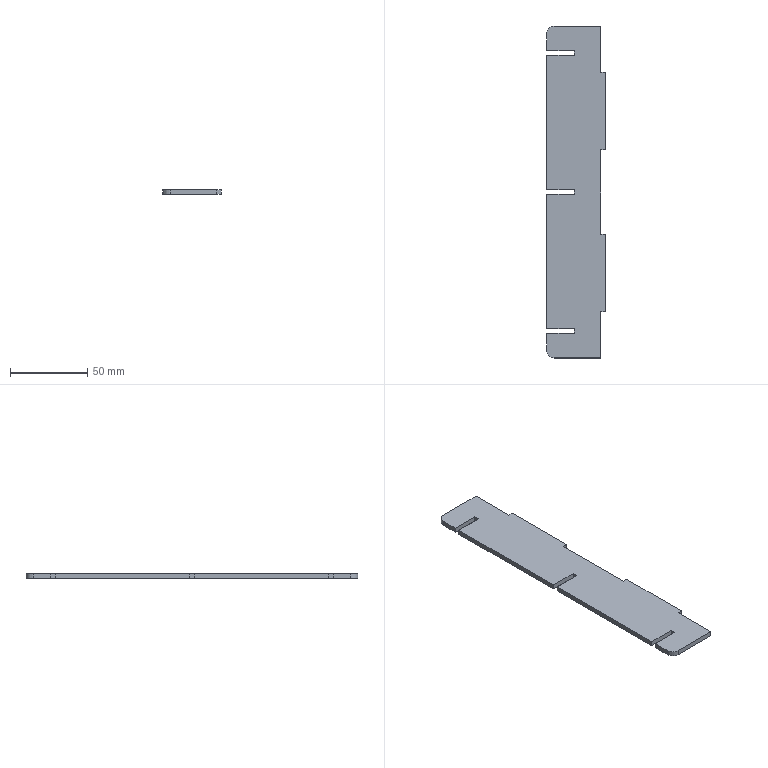Part | SolidWorks | features FlatPattern 1, SMBaseFlange 1, SheetMetal 1 | 1 solid | 28 faces | box 38 x 215 x 3.2 mm | volume 24453 mm3 | plane 26 | cylinder 2 | commonest cylinder face diameters 10 x2
STEP:
#1=CARTESIAN_POINT('',(-36.436,98.8,0.));
#2=VERTEX_POINT('',#1);
#3=CARTESIAN_POINT('',(-36.436,128.8,0.));
#4=VERTEX_POINT('',#3);
#5=CARTESIAN_POINT('',(-36.436,128.8,0.));
#6=DIRECTION('',(0.,1.,0.));
#7=VECTOR('',#6,1000.);
#8=LINE('',#5,#7);
#9=EDGE_CURVE('',#2,#4,#8,.T.);
#10=ORIENTED_EDGE('',*,*,#9,.F.);
#11=CARTESIAN_POINT('',(-36.436,98.8,-3.2));
#12=VERTEX_POINT('',#11);
#13=CARTESIAN_POINT('',(-36.436,98.8,-3.2));
#14=DIRECTION('',(0.,0.,1.));
#15=VECTOR('',#14,1000.);
#16=LINE('',#13,#15);
#17=EDGE_CURVE('',#12,#2,#16,.T.);
#18=ORIENTED_EDGE('',*,*,#17,.F.);
#19=CARTESIAN_POINT('',(-36.436,128.8,-3.2));
#20=VERTEX_POINT('',#19);
#21=CARTESIAN_POINT('',(-36.436,128.8,-3.2));
#22=DIRECTION('',(0.,1.,0.));
#23=VECTOR('',#22,1000.);
#24=LINE('',#21,#23);
#25=EDGE_CURVE('',#12,#20,#24,.T.);
#26=ORIENTED_EDGE('',*,*,#25,.T.);
#27=CARTESIAN_POINT('',(-36.436,128.8,-3.2));
#28=DIRECTION('',(0.,0.,1.));
#29=VECTOR('',#28,1000.);
#30=LINE('',#27,#29);
#31=EDGE_CURVE('',#20,#4,#30,.T.);
#32=ORIENTED_EDGE('',*,*,#31,.T.);
#33=EDGE_LOOP('',(#10,#18,#26,#32));
#34=FACE_OUTER_BOUND('',#33,.T.);
#35=CARTESIAN_POINT('',(-36.436,128.8,-3.2));
#36=DIRECTION('',(1.,0.,0.));
#37=DIRECTION('',(0.,1.,0.));
#38=AXIS2_PLACEMENT_3D('',#35,#36,#37);
#39=PLANE('',#38);
#40=ADVANCED_FACE('',(#34),#39,.T.);
#41=CARTESIAN_POINT('',(-33.436,98.8,0.));
#42=VERTEX_POINT('',#41);
#43=CARTESIAN_POINT('',(-36.436,98.8,0.));
#44=DIRECTION('',(-1.,0.,0.));
#45=VECTOR('',#44,1000.);
#46=LINE('',#43,#45);
#47=EDGE_CURVE('',#42,#2,#46,.T.);
#48=ORIENTED_EDGE('',*,*,#47,.F.);
#49=CARTESIAN_POINT('',(-33.436,98.8,-3.2));
#50=VERTEX_POINT('',#49);
#51=CARTESIAN_POINT('',(-33.436,98.8,-3.2));
#52=DIRECTION('',(0.,0.,1.));
#53=VECTOR('',#52,1000.);
#54=LINE('',#51,#53);
#55=EDGE_CURVE('',#50,#42,#54,.T.);
#56=ORIENTED_EDGE('',*,*,#55,.F.);
#57=CARTESIAN_POINT('',(-36.436,98.8,-3.2));
#58=DIRECTION('',(-1.,0.,0.));
#59=VECTOR('',#58,1000.);
#60=LINE('',#57,#59);
#61=EDGE_CURVE('',#50,#12,#60,.T.);
#62=ORIENTED_EDGE('',*,*,#61,.T.);
#63=ORIENTED_EDGE('',*,*,#17,.T.);
#64=EDGE_LOOP('',(#48,#56,#62,#63));
#65=FACE_OUTER_BOUND('',#64,.T.);
#66=CARTESIAN_POINT('',(-36.436,98.8,-3.2));
#67=DIRECTION('',(0.,1.,0.));
#68=DIRECTION('',(0.,0.,1.));
#69=AXIS2_PLACEMENT_3D('',#66,#67,#68);
#70=PLANE('',#69);
#71=ADVANCED_FACE('',(#65),#70,.T.);
#72=CARTESIAN_POINT('',(-33.436,48.8,0.));
#73=VERTEX_POINT('',#72);
#74=CARTESIAN_POINT('',(-33.436,98.8,0.));
#75=DIRECTION('',(0.,1.,0.));
#76=VECTOR('',#75,1000.);
#77=LINE('',#74,#76);
#78=EDGE_CURVE('',#73,#42,#77,.T.);
#79=ORIENTED_EDGE('',*,*,#78,.F.);
#80=CARTESIAN_POINT('',(-33.436,48.8,-3.2));
#81=VERTEX_POINT('',#80);
#82=CARTESIAN_POINT('',(-33.436,48.8,-3.2));
#83=DIRECTION('',(0.,0.,1.));
#84=VECTOR('',#83,1000.);
#85=LINE('',#82,#84);
#86=EDGE_CURVE('',#81,#73,#85,.T.);
#87=ORIENTED_EDGE('',*,*,#86,.F.);
#88=CARTESIAN_POINT('',(-33.436,98.8,-3.2));
#89=DIRECTION('',(0.,1.,0.));
#90=VECTOR('',#89,1000.);
#91=LINE('',#88,#90);
#92=EDGE_CURVE('',#81,#50,#91,.T.);
#93=ORIENTED_EDGE('',*,*,#92,.T.);
#94=ORIENTED_EDGE('',*,*,#55,.T.);
#95=EDGE_LOOP('',(#79,#87,#93,#94));
#96=FACE_OUTER_BOUND('',#95,.T.);
#97=CARTESIAN_POINT('',(-33.436,98.8,-3.2));
#98=DIRECTION('',(1.,0.,0.));
#99=DIRECTION('',(0.,1.,0.));
#100=AXIS2_PLACEMENT_3D('',#97,#98,#99);
#101=PLANE('',#100);
#102=ADVANCED_FACE('',(#96),#101,.T.);
#103=CARTESIAN_POINT('',(-36.436,48.8,0.));
#104=VERTEX_POINT('',#103);
#105=CARTESIAN_POINT('',(-33.436,48.8,0.));
#106=DIRECTION('',(1.,0.,0.));
#107=VECTOR('',#106,1000.);
#108=LINE('',#105,#107);
#109=EDGE_CURVE('',#104,#73,#108,.T.);
#110=ORIENTED_EDGE('',*,*,#109,.F.);
#111=CARTESIAN_POINT('',(-36.436,48.8,-3.2));
#112=VERTEX_POINT('',#111);
#113=CARTESIAN_POINT('',(-36.436,48.8,-3.2));
#114=DIRECTION('',(0.,0.,1.));
#115=VECTOR('',#114,1000.);
#116=LINE('',#113,#115);
#117=EDGE_CURVE('',#112,#104,#116,.T.);
#118=ORIENTED_EDGE('',*,*,#117,.F.);
#119=CARTESIAN_POINT('',(-33.436,48.8,-3.2));
#120=DIRECTION('',(1.,0.,0.));
#121=VECTOR('',#120,1000.);
#122=LINE('',#119,#121);
#123=EDGE_CURVE('',#112,#81,#122,.T.);
#124=ORIENTED_EDGE('',*,*,#123,.T.);
#125=ORIENTED_EDGE('',*,*,#86,.T.);
#126=EDGE_LOOP('',(#110,#118,#124,#125));
#127=FACE_OUTER_BOUND('',#126,.T.);
#128=CARTESIAN_POINT('',(-33.436,48.8,-3.2));
#129=DIRECTION('',(0.,-1.,0.));
#130=DIRECTION('',(0.,0.,-1.));
#131=AXIS2_PLACEMENT_3D('',#128,#129,#130);
#132=PLANE('',#131);
#133=ADVANCED_FACE('',(#127),#132,.T.);
#134=CARTESIAN_POINT('',(-36.436,-6.2,0.));
#135=VERTEX_POINT('',#134);
#136=CARTESIAN_POINT('',(-36.436,48.8,0.));
#137=DIRECTION('',(0.,1.,0.));
#138=VECTOR('',#137,1000.);
#139=LINE('',#136,#138);
#140=EDGE_CURVE('',#135,#104,#139,.T.);
#141=ORIENTED_EDGE('',*,*,#140,.F.);
#142=CARTESIAN_POINT('',(-36.436,-6.2,-3.2));
#143=VERTEX_POINT('',#142);
#144=CARTESIAN_POINT('',(-36.436,-6.2,-3.2));
#145=DIRECTION('',(0.,0.,1.));
#146=VECTOR('',#145,1000.);
#147=LINE('',#144,#146);
#148=EDGE_CURVE('',#143,#135,#147,.T.);
#149=ORIENTED_EDGE('',*,*,#148,.F.);
#150=CARTESIAN_POINT('',(-36.436,48.8,-3.2));
#151=DIRECTION('',(0.,1.,0.));
#152=VECTOR('',#151,1000.);
#153=LINE('',#150,#152);
#154=EDGE_CURVE('',#143,#112,#153,.T.);
#155=ORIENTED_EDGE('',*,*,#154,.T.);
#156=ORIENTED_EDGE('',*,*,#117,.T.);
#157=EDGE_LOOP('',(#141,#149,#155,#156));
#158=FACE_OUTER_BOUND('',#157,.T.);
#159=CARTESIAN_POINT('',(-36.436,48.8,-3.2));
#160=DIRECTION('',(1.,0.,0.));
#161=DIRECTION('',(0.,1.,0.));
#162=AXIS2_PLACEMENT_3D('',#159,#160,#161);
#163=PLANE('',#162);
#164=ADVANCED_FACE('',(#158),#163,.T.);
#165=CARTESIAN_POINT('',(-33.436,-6.2,0.));
#166=VERTEX_POINT('',#165);
#167=CARTESIAN_POINT('',(-33.436,-6.2,0.));
#168=DIRECTION('',(-1.,0.,0.));
#169=VECTOR('',#168,1000.);
#170=LINE('',#167,#169);
#171=EDGE_CURVE('',#166,#135,#170,.T.);
#172=ORIENTED_EDGE('',*,*,#171,.F.);
#173=CARTESIAN_POINT('',(-33.436,-6.2,-3.2));
#174=VERTEX_POINT('',#173);
#175=CARTESIAN_POINT('',(-33.436,-6.2,-3.2));
#176=DIRECTION('',(0.,0.,1.));
#177=VECTOR('',#176,1000.);
#178=LINE('',#175,#177);
#179=EDGE_CURVE('',#174,#166,#178,.T.);
#180=ORIENTED_EDGE('',*,*,#179,.F.);
#181=CARTESIAN_POINT('',(-33.436,-6.2,-3.2));
#182=DIRECTION('',(-1.,0.,0.));
#183=VECTOR('',#182,1000.);
#184=LINE('',#181,#183);
#185=EDGE_CURVE('',#174,#143,#184,.T.);
#186=ORIENTED_EDGE('',*,*,#185,.T.);
#187=ORIENTED_EDGE('',*,*,#148,.T.);
#188=EDGE_LOOP('',(#172,#180,#186,#187));
#189=FACE_OUTER_BOUND('',#188,.T.);
#190=CARTESIAN_POINT('',(-33.436,-6.2,-3.2));
#191=DIRECTION('',(0.,1.,0.));
#192=DIRECTION('',(-1.,0.,0.));
#193=AXIS2_PLACEMENT_3D('',#190,#191,#192);
#194=PLANE('',#193);
#195=ADVANCED_FACE('',(#189),#194,.T.);
#196=CARTESIAN_POINT('',(-33.436,-56.2,0.));
#197=VERTEX_POINT('',#196);
#198=CARTESIAN_POINT('',(-33.436,-56.2,0.));
#199=DIRECTION('',(0.,1.,0.));
#200=VECTOR('',#199,1000.);
#201=LINE('',#198,#200);
#202=EDGE_CURVE('',#197,#166,#201,.T.);
#203=ORIENTED_EDGE('',*,*,#202,.F.);
#204=CARTESIAN_POINT('',(-33.436,-56.2,-3.2));
#205=VERTEX_POINT('',#204);
#206=CARTESIAN_POINT('',(-33.436,-56.2,-3.2));
#207=DIRECTION('',(0.,0.,1.));
#208=VECTOR('',#207,1000.);
#209=LINE('',#206,#208);
#210=EDGE_CURVE('',#205,#197,#209,.T.);
#211=ORIENTED_EDGE('',*,*,#210,.F.);
#212=CARTESIAN_POINT('',(-33.436,-56.2,-3.2));
#213=DIRECTION('',(0.,1.,0.));
#214=VECTOR('',#213,1000.);
#215=LINE('',#212,#214);
#216=EDGE_CURVE('',#205,#174,#215,.T.);
#217=ORIENTED_EDGE('',*,*,#216,.T.);
#218=ORIENTED_EDGE('',*,*,#179,.T.);
#219=EDGE_LOOP('',(#203,#211,#217,#218));
#220=FACE_OUTER_BOUND('',#219,.T.);
#221=CARTESIAN_POINT('',(-33.436,-56.2,-3.2));
#222=DIRECTION('',(1.,0.,0.));
#223=DIRECTION('',(0.,1.,0.));
#224=AXIS2_PLACEMENT_3D('',#221,#222,#223);
#225=PLANE('',#224);
#226=ADVANCED_FACE('',(#220),#225,.T.);
#227=CARTESIAN_POINT('',(-36.436,-56.2,0.));
#228=VERTEX_POINT('',#227);
#229=CARTESIAN_POINT('',(-36.436,-56.2,0.));
#230=DIRECTION('',(1.,0.,0.));
#231=VECTOR('',#230,1000.);
#232=LINE('',#229,#231);
#233=EDGE_CURVE('',#228,#197,#232,.T.);
#234=ORIENTED_EDGE('',*,*,#233,.F.);
#235=CARTESIAN_POINT('',(-36.436,-56.2,-3.2));
#236=VERTEX_POINT('',#235);
#237=CARTESIAN_POINT('',(-36.436,-56.2,-3.2));
#238=DIRECTION('',(0.,0.,1.));
#239=VECTOR('',#238,1000.);
#240=LINE('',#237,#239);
#241=EDGE_CURVE('',#236,#228,#240,.T.);
#242=ORIENTED_EDGE('',*,*,#241,.F.);
#243=CARTESIAN_POINT('',(-36.436,-56.2,-3.2));
#244=DIRECTION('',(1.,0.,0.));
#245=VECTOR('',#244,1000.);
#246=LINE('',#243,#245);
#247=EDGE_CURVE('',#236,#205,#246,.T.);
#248=ORIENTED_EDGE('',*,*,#247,.T.);
#249=ORIENTED_EDGE('',*,*,#210,.T.);
#250=EDGE_LOOP('',(#234,#242,#248,#249));
#251=FACE_OUTER_BOUND('',#250,.T.);
#252=CARTESIAN_POINT('',(-36.436,-56.2,-3.2));
#253=DIRECTION('',(0.,-1.,0.));
#254=DIRECTION('',(0.,0.,-1.));
#255=AXIS2_PLACEMENT_3D('',#252,#253,#254);
#256=PLANE('',#255);
#257=ADVANCED_FACE('',(#251),#256,.T.);
#258=CARTESIAN_POINT('',(-36.436,-86.2,0.));
#259=VERTEX_POINT('',#258);
#260=CARTESIAN_POINT('',(-36.436,-56.2,0.));
#261=DIRECTION('',(0.,1.,0.));
#262=VECTOR('',#261,1000.);
#263=LINE('',#260,#262);
#264=EDGE_CURVE('',#259,#228,#263,.T.);
#265=ORIENTED_EDGE('',*,*,#264,.F.);
#266=CARTESIAN_POINT('',(-36.436,-86.2,-3.2));
#267=VERTEX_POINT('',#266);
#268=CARTESIAN_POINT('',(-36.436,-86.2,-3.2));
#269=DIRECTION('',(0.,0.,1.));
#270=VECTOR('',#269,1000.);
#271=LINE('',#268,#270);
#272=EDGE_CURVE('',#267,#259,#271,.T.);
#273=ORIENTED_EDGE('',*,*,#272,.F.);
#274=CARTESIAN_POINT('',(-36.436,-56.2,-3.2));
#275=DIRECTION('',(0.,1.,0.));
#276=VECTOR('',#275,1000.);
#277=LINE('',#274,#276);
#278=EDGE_CURVE('',#267,#236,#277,.T.);
#279=ORIENTED_EDGE('',*,*,#278,.T.);
#280=ORIENTED_EDGE('',*,*,#241,.T.);
#281=EDGE_LOOP('',(#265,#273,#279,#280));
#282=FACE_OUTER_BOUND('',#281,.T.);
#283=CARTESIAN_POINT('',(-36.436,-56.2,-3.2));
#284=DIRECTION('',(1.,0.,0.));
#285=DIRECTION('',(0.,1.,0.));
#286=AXIS2_PLACEMENT_3D('',#283,#284,#285);
#287=PLANE('',#286);
#288=ADVANCED_FACE('',(#282),#287,.T.);
#289=CARTESIAN_POINT('',(-66.436,-86.2,0.));
#290=VERTEX_POINT('',#289);
#291=CARTESIAN_POINT('',(-36.436,-86.2,0.));
#292=DIRECTION('',(1.,0.,0.));
#293=VECTOR('',#292,1000.);
#294=LINE('',#291,#293);
#295=EDGE_CURVE('',#290,#259,#294,.T.);
#296=ORIENTED_EDGE('',*,*,#295,.F.);
#297=CARTESIAN_POINT('',(-66.436,-86.2,-3.2));
#298=VERTEX_POINT('',#297);
#299=CARTESIAN_POINT('',(-66.436,-86.2,-3.2));
#300=DIRECTION('',(0.,0.,1.));
#301=VECTOR('',#300,1000.);
#302=LINE('',#299,#301);
#303=EDGE_CURVE('',#298,#290,#302,.T.);
#304=ORIENTED_EDGE('',*,*,#303,.F.);
#305=CARTESIAN_POINT('',(-36.436,-86.2,-3.2));
#306=DIRECTION('',(1.,0.,0.));
#307=VECTOR('',#306,1000.);
#308=LINE('',#305,#307);
#309=EDGE_CURVE('',#298,#267,#308,.T.);
#310=ORIENTED_EDGE('',*,*,#309,.T.);
#311=ORIENTED_EDGE('',*,*,#272,.T.);
#312=EDGE_LOOP('',(#296,#304,#310,#311));
#313=FACE_OUTER_BOUND('',#312,.T.);
#314=CARTESIAN_POINT('',(-36.436,-86.2,-3.2));
#315=DIRECTION('',(0.,-1.,0.));
#316=DIRECTION('',(0.,0.,-1.));
#317=AXIS2_PLACEMENT_3D('',#314,#315,#316);
#318=PLANE('',#317);
#319=ADVANCED_FACE('',(#313),#318,.T.);
#320=CARTESIAN_POINT('',(-71.436,-81.2,0.));
#321=VERTEX_POINT('',#320);
#322=CARTESIAN_POINT('',(-66.436,-81.2,0.));
#323=DIRECTION('',(0.,0.,1.));
#324=DIRECTION('',(-1.,0.,0.));
#325=AXIS2_PLACEMENT_3D('',#322,#323,#324);
#326=CIRCLE('',#325,5.);
#327=EDGE_CURVE('',#321,#290,#326,.T.);
#328=ORIENTED_EDGE('',*,*,#327,.F.);
#329=CARTESIAN_POINT('',(-71.436,-81.2,-3.2));
#330=VERTEX_POINT('',#329);
#331=CARTESIAN_POINT('',(-71.436,-81.2,-3.2));
#332=DIRECTION('',(0.,0.,1.));
#333=VECTOR('',#332,1000.);
#334=LINE('',#331,#333);
#335=EDGE_CURVE('',#330,#321,#334,.T.);
#336=ORIENTED_EDGE('',*,*,#335,.F.);
#337=CARTESIAN_POINT('',(-66.436,-81.2,-3.2));
#338=DIRECTION('',(0.,0.,1.));
#339=DIRECTION('',(-1.,0.,0.));
#340=AXIS2_PLACEMENT_3D('',#337,#338,#339);
#341=CIRCLE('',#340,5.);
#342=EDGE_CURVE('',#330,#298,#341,.T.);
#343=ORIENTED_EDGE('',*,*,#342,.T.);
#344=ORIENTED_EDGE('',*,*,#303,.T.);
#345=EDGE_LOOP('',(#328,#336,#343,#344));
#346=FACE_OUTER_BOUND('',#345,.T.);
#347=CARTESIAN_POINT('',(-66.436,-81.2,-3.2));
#348=DIRECTION('',(0.,0.,1.));
#349=DIRECTION('',(1.,0.,0.));
#350=AXIS2_PLACEMENT_3D('',#347,#348,#349);
#351=CYLINDRICAL_SURFACE('',#350,5.);
#352=ADVANCED_FACE('',(#346),#351,.T.);
#353=CARTESIAN_POINT('',(-71.436,-70.3,0.));
#354=VERTEX_POINT('',#353);
#355=CARTESIAN_POINT('',(-71.436,-70.3,0.));
#356=DIRECTION('',(0.,-1.,0.));
#357=VECTOR('',#356,1000.);
#358=LINE('',#355,#357);
#359=EDGE_CURVE('',#354,#321,#358,.T.);
#360=ORIENTED_EDGE('',*,*,#359,.F.);
#361=CARTESIAN_POINT('',(-71.436,-70.3,-3.2));
#362=VERTEX_POINT('',#361);
#363=CARTESIAN_POINT('',(-71.436,-70.3,-3.2));
#364=DIRECTION('',(0.,0.,1.));
#365=VECTOR('',#364,1000.);
#366=LINE('',#363,#365);
#367=EDGE_CURVE('',#362,#354,#366,.T.);
#368=ORIENTED_EDGE('',*,*,#367,.F.);
#369=CARTESIAN_POINT('',(-71.436,-70.3,-3.2));
#370=DIRECTION('',(0.,-1.,0.));
#371=VECTOR('',#370,1000.);
#372=LINE('',#369,#371);
#373=EDGE_CURVE('',#362,#330,#372,.T.);
#374=ORIENTED_EDGE('',*,*,#373,.T.);
#375=ORIENTED_EDGE('',*,*,#335,.T.);
#376=EDGE_LOOP('',(#360,#368,#374,#375));
#377=FACE_OUTER_BOUND('',#376,.T.);
#378=CARTESIAN_POINT('',(-71.436,-70.3,-3.2));
#379=DIRECTION('',(-1.,0.,0.));
#380=DIRECTION('',(0.,-1.,0.));
#381=AXIS2_PLACEMENT_3D('',#378,#379,#380);
#382=PLANE('',#381);
#383=ADVANCED_FACE('',(#377),#382,.T.);
#384=CARTESIAN_POINT('',(-53.436,-70.3,0.));
#385=VERTEX_POINT('',#384);
#386=CARTESIAN_POINT('',(-53.436,-70.3,0.));
#387=DIRECTION('',(-1.,0.,0.));
#388=VECTOR('',#387,1000.);
#389=LINE('',#386,#388);
#390=EDGE_CURVE('',#385,#354,#389,.T.);
#391=ORIENTED_EDGE('',*,*,#390,.F.);
#392=CARTESIAN_POINT('',(-53.436,-70.3,-3.2));
#393=VERTEX_POINT('',#392);
#394=CARTESIAN_POINT('',(-53.436,-70.3,-3.2));
#395=DIRECTION('',(0.,0.,1.));
#396=VECTOR('',#395,1000.);
#397=LINE('',#394,#396);
#398=EDGE_CURVE('',#393,#385,#397,.T.);
#399=ORIENTED_EDGE('',*,*,#398,.F.);
#400=CARTESIAN_POINT('',(-53.436,-70.3,-3.2));
#401=DIRECTION('',(-1.,0.,0.));
#402=VECTOR('',#401,1000.);
#403=LINE('',#400,#402);
#404=EDGE_CURVE('',#393,#362,#403,.T.);
#405=ORIENTED_EDGE('',*,*,#404,.T.);
#406=ORIENTED_EDGE('',*,*,#367,.T.);
#407=EDGE_LOOP('',(#391,#399,#405,#406));
#408=FACE_OUTER_BOUND('',#407,.T.);
#409=CARTESIAN_POINT('',(-53.436,-70.3,-3.2));
#410=DIRECTION('',(0.,1.,0.));
#411=DIRECTION('',(-1.,0.,0.));
#412=AXIS2_PLACEMENT_3D('',#409,#410,#411);
#413=PLANE('',#412);
#414=ADVANCED_FACE('',(#408),#413,.T.);
#415=CARTESIAN_POINT('',(-53.436,-67.1,0.));
#416=VERTEX_POINT('',#415);
#417=CARTESIAN_POINT('',(-53.436,-67.1,0.));
#418=DIRECTION('',(0.,-1.,0.));
#419=VECTOR('',#418,1000.);
#420=LINE('',#417,#419);
#421=EDGE_CURVE('',#416,#385,#420,.T.);
#422=ORIENTED_EDGE('',*,*,#421,.F.);
#423=CARTESIAN_POINT('',(-53.436,-67.1,-3.2));
#424=VERTEX_POINT('',#423);
#425=CARTESIAN_POINT('',(-53.436,-67.1,-3.2));
#426=DIRECTION('',(0.,0.,1.));
#427=VECTOR('',#426,1000.);
#428=LINE('',#425,#427);
#429=EDGE_CURVE('',#424,#416,#428,.T.);
#430=ORIENTED_EDGE('',*,*,#429,.F.);
#431=CARTESIAN_POINT('',(-53.436,-67.1,-3.2));
#432=DIRECTION('',(0.,-1.,0.));
#433=VECTOR('',#432,1000.);
#434=LINE('',#431,#433);
#435=EDGE_CURVE('',#424,#393,#434,.T.);
#436=ORIENTED_EDGE('',*,*,#435,.T.);
#437=ORIENTED_EDGE('',*,*,#398,.T.);
#438=EDGE_LOOP('',(#422,#430,#436,#437));
#439=FACE_OUTER_BOUND('',#438,.T.);
#440=CARTESIAN_POINT('',(-53.436,-67.1,-3.2));
#441=DIRECTION('',(-1.,0.,0.));
#442=DIRECTION('',(0.,0.,1.));
#443=AXIS2_PLACEMENT_3D('',#440,#441,#442);
#444=PLANE('',#443);
#445=ADVANCED_FACE('',(#439),#444,.T.);
#446=CARTESIAN_POINT('',(-71.436,-67.1,0.));
#447=VERTEX_POINT('',#446);
#448=CARTESIAN_POINT('',(-71.436,-67.1,0.));
#449=DIRECTION('',(1.,0.,0.));
#450=VECTOR('',#449,1000.);
#451=LINE('',#448,#450);
#452=EDGE_CURVE('',#447,#416,#451,.T.);
#453=ORIENTED_EDGE('',*,*,#452,.F.);
#454=CARTESIAN_POINT('',(-71.436,-67.1,-3.2));
#455=VERTEX_POINT('',#454);
#456=CARTESIAN_POINT('',(-71.436,-67.1,-3.2));
#457=DIRECTION('',(0.,0.,1.));
#458=VECTOR('',#457,1000.);
#459=LINE('',#456,#458);
#460=EDGE_CURVE('',#455,#447,#459,.T.);
#461=ORIENTED_EDGE('',*,*,#460,.F.);
#462=CARTESIAN_POINT('',(-71.436,-67.1,-3.2));
#463=DIRECTION('',(1.,0.,0.));
#464=VECTOR('',#463,1000.);
#465=LINE('',#462,#464);
#466=EDGE_CURVE('',#455,#424,#465,.T.);
#467=ORIENTED_EDGE('',*,*,#466,.T.);
#468=ORIENTED_EDGE('',*,*,#429,.T.);
#469=EDGE_LOOP('',(#453,#461,#467,#468));
#470=FACE_OUTER_BOUND('',#469,.T.);
#471=CARTESIAN_POINT('',(-71.436,-67.1,-3.2));
#472=DIRECTION('',(0.,-1.,0.));
#473=DIRECTION('',(1.,0.,0.));
#474=AXIS2_PLACEMENT_3D('',#471,#472,#473);
#475=PLANE('',#474);
#476=ADVANCED_FACE('',(#470),#475,.T.);
#477=CARTESIAN_POINT('',(-71.436,19.7,0.));
#478=VERTEX_POINT('',#477);
#479=CARTESIAN_POINT('',(-71.436,19.7,0.));
#480=DIRECTION('',(0.,-1.,0.));
#481=VECTOR('',#480,1000.);
#482=LINE('',#479,#481);
#483=EDGE_CURVE('',#478,#447,#482,.T.);
#484=ORIENTED_EDGE('',*,*,#483,.F.);
#485=CARTESIAN_POINT('',(-71.436,19.7,-3.2));
#486=VERTEX_POINT('',#485);
#487=CARTESIAN_POINT('',(-71.436,19.7,-3.2));
#488=DIRECTION('',(0.,0.,1.));
#489=VECTOR('',#488,1000.);
#490=LINE('',#487,#489);
#491=EDGE_CURVE('',#486,#478,#490,.T.);
#492=ORIENTED_EDGE('',*,*,#491,.F.);
#493=CARTESIAN_POINT('',(-71.436,19.7,-3.2));
#494=DIRECTION('',(0.,-1.,0.));
#495=VECTOR('',#494,1000.);
#496=LINE('',#493,#495);
#497=EDGE_CURVE('',#486,#455,#496,.T.);
#498=ORIENTED_EDGE('',*,*,#497,.T.);
#499=ORIENTED_EDGE('',*,*,#460,.T.);
#500=EDGE_LOOP('',(#484,#492,#498,#499));
#501=FACE_OUTER_BOUND('',#500,.T.);
#502=CARTESIAN_POINT('',(-71.436,19.7,-3.2));
#503=DIRECTION('',(-1.,0.,0.));
#504=DIRECTION('',(0.,-1.,0.));
#505=AXIS2_PLACEMENT_3D('',#502,#503,#504);
#506=PLANE('',#505);
#507=ADVANCED_FACE('',(#501),#506,.T.);
#508=CARTESIAN_POINT('',(-53.436,19.7,0.));
#509=VERTEX_POINT('',#508);
#510=CARTESIAN_POINT('',(-53.436,19.7,0.));
#511=DIRECTION('',(-1.,0.,0.));
#512=VECTOR('',#511,1000.);
#513=LINE('',#510,#512);
#514=EDGE_CURVE('',#509,#478,#513,.T.);
#515=ORIENTED_EDGE('',*,*,#514,.F.);
#516=CARTESIAN_POINT('',(-53.436,19.7,-3.2));
#517=VERTEX_POINT('',#516);
#518=CARTESIAN_POINT('',(-53.436,19.7,-3.2));
#519=DIRECTION('',(0.,0.,1.));
#520=VECTOR('',#519,1000.);
#521=LINE('',#518,#520);
#522=EDGE_CURVE('',#517,#509,#521,.T.);
#523=ORIENTED_EDGE('',*,*,#522,.F.);
#524=CARTESIAN_POINT('',(-53.436,19.7,-3.2));
#525=DIRECTION('',(-1.,0.,0.));
#526=VECTOR('',#525,1000.);
#527=LINE('',#524,#526);
#528=EDGE_CURVE('',#517,#486,#527,.T.);
#529=ORIENTED_EDGE('',*,*,#528,.T.);
#530=ORIENTED_EDGE('',*,*,#491,.T.);
#531=EDGE_LOOP('',(#515,#523,#529,#530));
#532=FACE_OUTER_BOUND('',#531,.T.);
#533=CARTESIAN_POINT('',(-53.436,19.7,-3.2));
#534=DIRECTION('',(0.,1.,0.));
#535=DIRECTION('',(-1.,0.,0.));
#536=AXIS2_PLACEMENT_3D('',#533,#534,#535);
#537=PLANE('',#536);
#538=ADVANCED_FACE('',(#532),#537,.T.);
#539=CARTESIAN_POINT('',(-53.436,22.9,0.));
#540=VERTEX_POINT('',#539);
#541=CARTESIAN_POINT('',(-53.436,22.9,0.));
#542=DIRECTION('',(0.,-1.,0.));
#543=VECTOR('',#542,1000.);
#544=LINE('',#541,#543);
#545=EDGE_CURVE('',#540,#509,#544,.T.);
#546=ORIENTED_EDGE('',*,*,#545,.F.);
#547=CARTESIAN_POINT('',(-53.436,22.9,-3.2));
#548=VERTEX_POINT('',#547);
#549=CARTESIAN_POINT('',(-53.436,22.9,-3.2));
#550=DIRECTION('',(0.,0.,1.));
#551=VECTOR('',#550,1000.);
#552=LINE('',#549,#551);
#553=EDGE_CURVE('',#548,#540,#552,.T.);
#554=ORIENTED_EDGE('',*,*,#553,.F.);
#555=CARTESIAN_POINT('',(-53.436,22.9,-3.2));
#556=DIRECTION('',(0.,-1.,0.));
#557=VECTOR('',#556,1000.);
#558=LINE('',#555,#557);
#559=EDGE_CURVE('',#548,#517,#558,.T.);
#560=ORIENTED_EDGE('',*,*,#559,.T.);
#561=ORIENTED_EDGE('',*,*,#522,.T.);
#562=EDGE_LOOP('',(#546,#554,#560,#561));
#563=FACE_OUTER_BOUND('',#562,.T.);
#564=CARTESIAN_POINT('',(-53.436,22.9,-3.2));
#565=DIRECTION('',(-1.,0.,0.));
#566=DIRECTION('',(0.,0.,1.));
#567=AXIS2_PLACEMENT_3D('',#564,#565,#566);
#568=PLANE('',#567);
#569=ADVANCED_FACE('',(#563),#568,.T.);
#570=CARTESIAN_POINT('',(-71.436,22.9,0.));
#571=VERTEX_POINT('',#570);
#572=CARTESIAN_POINT('',(-71.436,22.9,0.));
#573=DIRECTION('',(1.,0.,0.));
#574=VECTOR('',#573,1000.);
#575=LINE('',#572,#574);
#576=EDGE_CURVE('',#571,#540,#575,.T.);
#577=ORIENTED_EDGE('',*,*,#576,.F.);
#578=CARTESIAN_POINT('',(-71.436,22.9,-3.2));
#579=VERTEX_POINT('',#578);
#580=CARTESIAN_POINT('',(-71.436,22.9,-3.2));
#581=DIRECTION('',(0.,0.,1.));
#582=VECTOR('',#581,1000.);
#583=LINE('',#580,#582);
#584=EDGE_CURVE('',#579,#571,#583,.T.);
#585=ORIENTED_EDGE('',*,*,#584,.F.);
#586=CARTESIAN_POINT('',(-71.436,22.9,-3.2));
#587=DIRECTION('',(1.,0.,0.));
#588=VECTOR('',#587,1000.);
#589=LINE('',#586,#588);
#590=EDGE_CURVE('',#579,#548,#589,.T.);
#591=ORIENTED_EDGE('',*,*,#590,.T.);
#592=ORIENTED_EDGE('',*,*,#553,.T.);
#593=EDGE_LOOP('',(#577,#585,#591,#592));
#594=FACE_OUTER_BOUND('',#593,.T.);
#595=CARTESIAN_POINT('',(-71.436,22.9,-3.2));
#596=DIRECTION('',(0.,-1.,0.));
#597=DIRECTION('',(1.,0.,0.));
#598=AXIS2_PLACEMENT_3D('',#595,#596,#597);
#599=PLANE('',#598);
#600=ADVANCED_FACE('',(#594),#599,.T.);
#601=CARTESIAN_POINT('',(-71.436,109.7,0.));
#602=VERTEX_POINT('',#601);
#603=CARTESIAN_POINT('',(-71.436,109.7,0.));
#604=DIRECTION('',(0.,-1.,0.));
#605=VECTOR('',#604,1000.);
#606=LINE('',#603,#605);
#607=EDGE_CURVE('',#602,#571,#606,.T.);
#608=ORIENTED_EDGE('',*,*,#607,.F.);
#609=CARTESIAN_POINT('',(-71.436,109.7,-3.2));
#610=VERTEX_POINT('',#609);
#611=CARTESIAN_POINT('',(-71.436,109.7,-3.2));
#612=DIRECTION('',(0.,0.,1.));
#613=VECTOR('',#612,1000.);
#614=LINE('',#611,#613);
#615=EDGE_CURVE('',#610,#602,#614,.T.);
#616=ORIENTED_EDGE('',*,*,#615,.F.);
#617=CARTESIAN_POINT('',(-71.436,109.7,-3.2));
#618=DIRECTION('',(0.,-1.,0.));
#619=VECTOR('',#618,1000.);
#620=LINE('',#617,#619);
#621=EDGE_CURVE('',#610,#579,#620,.T.);
#622=ORIENTED_EDGE('',*,*,#621,.T.);
#623=ORIENTED_EDGE('',*,*,#584,.T.);
#624=EDGE_LOOP('',(#608,#616,#622,#623));
#625=FACE_OUTER_BOUND('',#624,.T.);
#626=CARTESIAN_POINT('',(-71.436,109.7,-3.2));
#627=DIRECTION('',(-1.,0.,0.));
#628=DIRECTION('',(0.,-1.,0.));
#629=AXIS2_PLACEMENT_3D('',#626,#627,#628);
#630=PLANE('',#629);
#631=ADVANCED_FACE('',(#625),#630,.T.);
#632=CARTESIAN_POINT('',(-53.436,109.7,0.));
#633=VERTEX_POINT('',#632);
#634=CARTESIAN_POINT('',(-53.436,109.7,0.));
#635=DIRECTION('',(-1.,0.,0.));
#636=VECTOR('',#635,1000.);
#637=LINE('',#634,#636);
#638=EDGE_CURVE('',#633,#602,#637,.T.);
#639=ORIENTED_EDGE('',*,*,#638,.F.);
#640=CARTESIAN_POINT('',(-53.436,109.7,-3.2));
#641=VERTEX_POINT('',#640);
#642=CARTESIAN_POINT('',(-53.436,109.7,-3.2));
#643=DIRECTION('',(0.,0.,1.));
#644=VECTOR('',#643,1000.);
#645=LINE('',#642,#644);
#646=EDGE_CURVE('',#641,#633,#645,.T.);
#647=ORIENTED_EDGE('',*,*,#646,.F.);
#648=CARTESIAN_POINT('',(-53.436,109.7,-3.2));
#649=DIRECTION('',(-1.,0.,0.));
#650=VECTOR('',#649,1000.);
#651=LINE('',#648,#650);
#652=EDGE_CURVE('',#641,#610,#651,.T.);
#653=ORIENTED_EDGE('',*,*,#652,.T.);
#654=ORIENTED_EDGE('',*,*,#615,.T.);
#655=EDGE_LOOP('',(#639,#647,#653,#654));
#656=FACE_OUTER_BOUND('',#655,.T.);
#657=CARTESIAN_POINT('',(-53.436,109.7,-3.2));
#658=DIRECTION('',(0.,1.,0.));
#659=DIRECTION('',(-1.,0.,0.));
#660=AXIS2_PLACEMENT_3D('',#657,#658,#659);
#661=PLANE('',#660);
#662=ADVANCED_FACE('',(#656),#661,.T.);
#663=CARTESIAN_POINT('',(-53.436,112.9,0.));
#664=VERTEX_POINT('',#663);
#665=CARTESIAN_POINT('',(-53.436,112.9,0.));
#666=DIRECTION('',(0.,-1.,0.));
#667=VECTOR('',#666,1000.);
#668=LINE('',#665,#667);
#669=EDGE_CURVE('',#664,#633,#668,.T.);
#670=ORIENTED_EDGE('',*,*,#669,.F.);
#671=CARTESIAN_POINT('',(-53.436,112.9,-3.2));
#672=VERTEX_POINT('',#671);
#673=CARTESIAN_POINT('',(-53.436,112.9,-3.2));
#674=DIRECTION('',(0.,0.,1.));
#675=VECTOR('',#674,1000.);
#676=LINE('',#673,#675);
#677=EDGE_CURVE('',#672,#664,#676,.T.);
#678=ORIENTED_EDGE('',*,*,#677,.F.);
#679=CARTESIAN_POINT('',(-53.436,112.9,-3.2));
#680=DIRECTION('',(0.,-1.,0.));
#681=VECTOR('',#680,1000.);
#682=LINE('',#679,#681);
#683=EDGE_CURVE('',#672,#641,#682,.T.);
#684=ORIENTED_EDGE('',*,*,#683,.T.);
#685=ORIENTED_EDGE('',*,*,#646,.T.);
#686=EDGE_LOOP('',(#670,#678,#684,#685));
#687=FACE_OUTER_BOUND('',#686,.T.);
#688=CARTESIAN_POINT('',(-53.436,112.9,-3.2));
#689=DIRECTION('',(-1.,0.,0.));
#690=DIRECTION('',(0.,0.,1.));
#691=AXIS2_PLACEMENT_3D('',#688,#689,#690);
#692=PLANE('',#691);
#693=ADVANCED_FACE('',(#687),#692,.T.);
#694=CARTESIAN_POINT('',(-71.436,112.9,0.));
#695=VERTEX_POINT('',#694);
#696=CARTESIAN_POINT('',(-71.436,112.9,0.));
#697=DIRECTION('',(1.,0.,0.));
#698=VECTOR('',#697,1000.);
#699=LINE('',#696,#698);
#700=EDGE_CURVE('',#695,#664,#699,.T.);
#701=ORIENTED_EDGE('',*,*,#700,.F.);
#702=CARTESIAN_POINT('',(-71.436,112.9,-3.2));
#703=VERTEX_POINT('',#702);
#704=CARTESIAN_POINT('',(-71.436,112.9,-3.2));
#705=DIRECTION('',(0.,0.,1.));
#706=VECTOR('',#705,1000.);
#707=LINE('',#704,#706);
#708=EDGE_CURVE('',#703,#695,#707,.T.);
#709=ORIENTED_EDGE('',*,*,#708,.F.);
#710=CARTESIAN_POINT('',(-71.436,112.9,-3.2));
#711=DIRECTION('',(1.,0.,0.));
#712=VECTOR('',#711,1000.);
#713=LINE('',#710,#712);
#714=EDGE_CURVE('',#703,#672,#713,.T.);
#715=ORIENTED_EDGE('',*,*,#714,.T.);
#716=ORIENTED_EDGE('',*,*,#677,.T.);
#717=EDGE_LOOP('',(#701,#709,#715,#716));
#718=FACE_OUTER_BOUND('',#717,.T.);
#719=CARTESIAN_POINT('',(-71.436,112.9,-3.2));
#720=DIRECTION('',(0.,-1.,0.));
#721=DIRECTION('',(1.,0.,0.));
#722=AXIS2_PLACEMENT_3D('',#719,#720,#721);
#723=PLANE('',#722);
#724=ADVANCED_FACE('',(#718),#723,.T.);
#725=CARTESIAN_POINT('',(-71.436,123.8,0.));
#726=VERTEX_POINT('',#725);
#727=CARTESIAN_POINT('',(-71.436,123.8,0.));
#728=DIRECTION('',(0.,-1.,0.));
#729=VECTOR('',#728,1000.);
#730=LINE('',#727,#729);
#731=EDGE_CURVE('',#726,#695,#730,.T.);
#732=ORIENTED_EDGE('',*,*,#731,.F.);
#733=CARTESIAN_POINT('',(-71.436,123.8,-3.2));
#734=VERTEX_POINT('',#733);
#735=CARTESIAN_POINT('',(-71.436,123.8,-3.2));
#736=DIRECTION('',(0.,0.,1.));
#737=VECTOR('',#736,1000.);
#738=LINE('',#735,#737);
#739=EDGE_CURVE('',#734,#726,#738,.T.);
#740=ORIENTED_EDGE('',*,*,#739,.F.);
#741=CARTESIAN_POINT('',(-71.436,123.8,-3.2));
#742=DIRECTION('',(0.,-1.,0.));
#743=VECTOR('',#742,1000.);
#744=LINE('',#741,#743);
#745=EDGE_CURVE('',#734,#703,#744,.T.);
#746=ORIENTED_EDGE('',*,*,#745,.T.);
#747=ORIENTED_EDGE('',*,*,#708,.T.);
#748=EDGE_LOOP('',(#732,#740,#746,#747));
#749=FACE_OUTER_BOUND('',#748,.T.);
#750=CARTESIAN_POINT('',(-71.436,123.8,-3.2));
#751=DIRECTION('',(-1.,0.,0.));
#752=DIRECTION('',(0.,-1.,0.));
#753=AXIS2_PLACEMENT_3D('',#750,#751,#752);
#754=PLANE('',#753);
#755=ADVANCED_FACE('',(#749),#754,.T.);
#756=CARTESIAN_POINT('',(-66.436,128.8,0.));
#757=VERTEX_POINT('',#756);
#758=CARTESIAN_POINT('',(-66.436,123.8,0.));
#759=DIRECTION('',(0.,0.,1.));
#760=DIRECTION('',(1.,0.,0.));
#761=AXIS2_PLACEMENT_3D('',#758,#759,#760);
#762=CIRCLE('',#761,5.);
#763=EDGE_CURVE('',#757,#726,#762,.T.);
#764=ORIENTED_EDGE('',*,*,#763,.F.);
#765=CARTESIAN_POINT('',(-66.436,128.8,-3.2));
#766=VERTEX_POINT('',#765);
#767=CARTESIAN_POINT('',(-66.436,128.8,-3.2));
#768=DIRECTION('',(0.,0.,1.));
#769=VECTOR('',#768,1000.);
#770=LINE('',#767,#769);
#771=EDGE_CURVE('',#766,#757,#770,.T.);
#772=ORIENTED_EDGE('',*,*,#771,.F.);
#773=CARTESIAN_POINT('',(-66.436,123.8,-3.2));
#774=DIRECTION('',(0.,0.,1.));
#775=DIRECTION('',(1.,0.,0.));
#776=AXIS2_PLACEMENT_3D('',#773,#774,#775);
#777=CIRCLE('',#776,5.);
#778=EDGE_CURVE('',#766,#734,#777,.T.);
#779=ORIENTED_EDGE('',*,*,#778,.T.);
#780=ORIENTED_EDGE('',*,*,#739,.T.);
#781=EDGE_LOOP('',(#764,#772,#779,#780));
#782=FACE_OUTER_BOUND('',#781,.T.);
#783=CARTESIAN_POINT('',(-66.436,123.8,-3.2));
#784=DIRECTION('',(0.,0.,1.));
#785=DIRECTION('',(1.,0.,0.));
#786=AXIS2_PLACEMENT_3D('',#783,#784,#785);
#787=CYLINDRICAL_SURFACE('',#786,5.);
#788=ADVANCED_FACE('',(#782),#787,.T.);
#789=CARTESIAN_POINT('',(-36.436,128.8,0.));
#790=DIRECTION('',(-1.,0.,0.));
#791=VECTOR('',#790,1000.);
#792=LINE('',#789,#791);
#793=EDGE_CURVE('',#4,#757,#792,.T.);
#794=ORIENTED_EDGE('',*,*,#793,.F.);
#795=ORIENTED_EDGE('',*,*,#31,.F.);
#796=CARTESIAN_POINT('',(-36.436,128.8,-3.2));
#797=DIRECTION('',(-1.,0.,0.));
#798=VECTOR('',#797,1000.);
#799=LINE('',#796,#798);
#800=EDGE_CURVE('',#20,#766,#799,.T.);
#801=ORIENTED_EDGE('',*,*,#800,.T.);
#802=ORIENTED_EDGE('',*,*,#771,.T.);
#803=EDGE_LOOP('',(#794,#795,#801,#802));
#804=FACE_OUTER_BOUND('',#803,.T.);
#805=CARTESIAN_POINT('',(-36.436,128.8,-3.2));
#806=DIRECTION('',(0.,1.,0.));
#807=DIRECTION('',(0.,0.,1.));
#808=AXIS2_PLACEMENT_3D('',#805,#806,#807);
#809=PLANE('',#808);
#810=ADVANCED_FACE('',(#804),#809,.T.);
#811=ORIENTED_EDGE('',*,*,#25,.F.);
#812=ORIENTED_EDGE('',*,*,#61,.F.);
#813=ORIENTED_EDGE('',*,*,#92,.F.);
#814=ORIENTED_EDGE('',*,*,#123,.F.);
#815=ORIENTED_EDGE('',*,*,#154,.F.);
#816=ORIENTED_EDGE('',*,*,#185,.F.);
#817=ORIENTED_EDGE('',*,*,#216,.F.);
#818=ORIENTED_EDGE('',*,*,#247,.F.);
#819=ORIENTED_EDGE('',*,*,#278,.F.);
#820=ORIENTED_EDGE('',*,*,#309,.F.);
#821=ORIENTED_EDGE('',*,*,#342,.F.);
#822=ORIENTED_EDGE('',*,*,#373,.F.);
#823=ORIENTED_EDGE('',*,*,#404,.F.);
#824=ORIENTED_EDGE('',*,*,#435,.F.);
#825=ORIENTED_EDGE('',*,*,#466,.F.);
#826=ORIENTED_EDGE('',*,*,#497,.F.);
#827=ORIENTED_EDGE('',*,*,#528,.F.);
#828=ORIENTED_EDGE('',*,*,#559,.F.);
#829=ORIENTED_EDGE('',*,*,#590,.F.);
#830=ORIENTED_EDGE('',*,*,#621,.F.);
#831=ORIENTED_EDGE('',*,*,#652,.F.);
#832=ORIENTED_EDGE('',*,*,#683,.F.);
#833=ORIENTED_EDGE('',*,*,#714,.F.);
#834=ORIENTED_EDGE('',*,*,#745,.F.);
#835=ORIENTED_EDGE('',*,*,#778,.F.);
#836=ORIENTED_EDGE('',*,*,#800,.F.);
#837=EDGE_LOOP('',(#811,#812,#813,#814,#815,#816,#817,#818,#819,#820,#821,#822,#823,#824,#825,#826,#827,#828,#829,#830,#831,#832,#833,#834,#835,#836));
#838=FACE_OUTER_BOUND('',#837,.T.);
#839=CARTESIAN_POINT('',(-66.436,-81.2,-3.2));
#840=DIRECTION('',(0.,0.,-1.));
#841=DIRECTION('',(-1.,0.,0.));
#842=AXIS2_PLACEMENT_3D('',#839,#840,#841);
#843=PLANE('',#842);
#844=ADVANCED_FACE('',(#838),#843,.T.);
#845=ORIENTED_EDGE('',*,*,#9,.T.);
#846=ORIENTED_EDGE('',*,*,#793,.T.);
#847=ORIENTED_EDGE('',*,*,#763,.T.);
#848=ORIENTED_EDGE('',*,*,#731,.T.);
#849=ORIENTED_EDGE('',*,*,#700,.T.);
#850=ORIENTED_EDGE('',*,*,#669,.T.);
#851=ORIENTED_EDGE('',*,*,#638,.T.);
#852=ORIENTED_EDGE('',*,*,#607,.T.);
#853=ORIENTED_EDGE('',*,*,#576,.T.);
#854=ORIENTED_EDGE('',*,*,#545,.T.);
#855=ORIENTED_EDGE('',*,*,#514,.T.);
#856=ORIENTED_EDGE('',*,*,#483,.T.);
#857=ORIENTED_EDGE('',*,*,#452,.T.);
#858=ORIENTED_EDGE('',*,*,#421,.T.);
#859=ORIENTED_EDGE('',*,*,#390,.T.);
#860=ORIENTED_EDGE('',*,*,#359,.T.);
#861=ORIENTED_EDGE('',*,*,#327,.T.);
#862=ORIENTED_EDGE('',*,*,#295,.T.);
#863=ORIENTED_EDGE('',*,*,#264,.T.);
#864=ORIENTED_EDGE('',*,*,#233,.T.);
#865=ORIENTED_EDGE('',*,*,#202,.T.);
#866=ORIENTED_EDGE('',*,*,#171,.T.);
#867=ORIENTED_EDGE('',*,*,#140,.T.);
#868=ORIENTED_EDGE('',*,*,#109,.T.);
#869=ORIENTED_EDGE('',*,*,#78,.T.);
#870=ORIENTED_EDGE('',*,*,#47,.T.);
#871=EDGE_LOOP('',(#845,#846,#847,#848,#849,#850,#851,#852,#853,#854,#855,#856,#857,#858,#859,#860,#861,#862,#863,#864,#865,#866,#867,#868,#869,#870));
#872=FACE_OUTER_BOUND('',#871,.T.);
#873=CARTESIAN_POINT('',(-66.436,-81.2,0.));
#874=DIRECTION('',(0.,0.,-1.));
#875=DIRECTION('',(-1.,0.,0.));
#876=AXIS2_PLACEMENT_3D('',#873,#874,#875);
#877=PLANE('',#876);
#878=ADVANCED_FACE('',(#872),#877,.F.);
#879=CLOSED_SHELL('',(#40,#71,#102,#133,#164,#195,#226,#257,#288,#319,#352,#383,#414,#445,#476,#507,#538,#569,#600,#631,#662,#693,#724,#755,#788,#810,#844,#878));
#880=MANIFOLD_SOLID_BREP('',#879);
#881=CARTESIAN_POINT('',(0.,0.,0.));
#882=DIRECTION('',(0.,0.,1.));
#883=DIRECTION('',(1.,0.,0.));
#884=AXIS2_PLACEMENT_3D('',#881,#882,#883);
#885=(LENGTH_UNIT()NAMED_UNIT(*)SI_UNIT(.MILLI.,.METRE.));
#886=UNCERTAINTY_MEASURE_WITH_UNIT(LENGTH_MEASURE(0.00001),#885,'','');
#887=(NAMED_UNIT(*)PLANE_ANGLE_UNIT()SI_UNIT($,.RADIAN.));
#888=(NAMED_UNIT(*)SI_UNIT($,.STERADIAN.)SOLID_ANGLE_UNIT());
#889=(GEOMETRIC_REPRESENTATION_CONTEXT(3)GLOBAL_UNCERTAINTY_ASSIGNED_CONTEXT((#886))GLOBAL_UNIT_ASSIGNED_CONTEXT((#885,#887,#888))REPRESENTATION_CONTEXT('',''));
#890=ADVANCED_BREP_SHAPE_REPRESENTATION('',(#880,#884),#889);